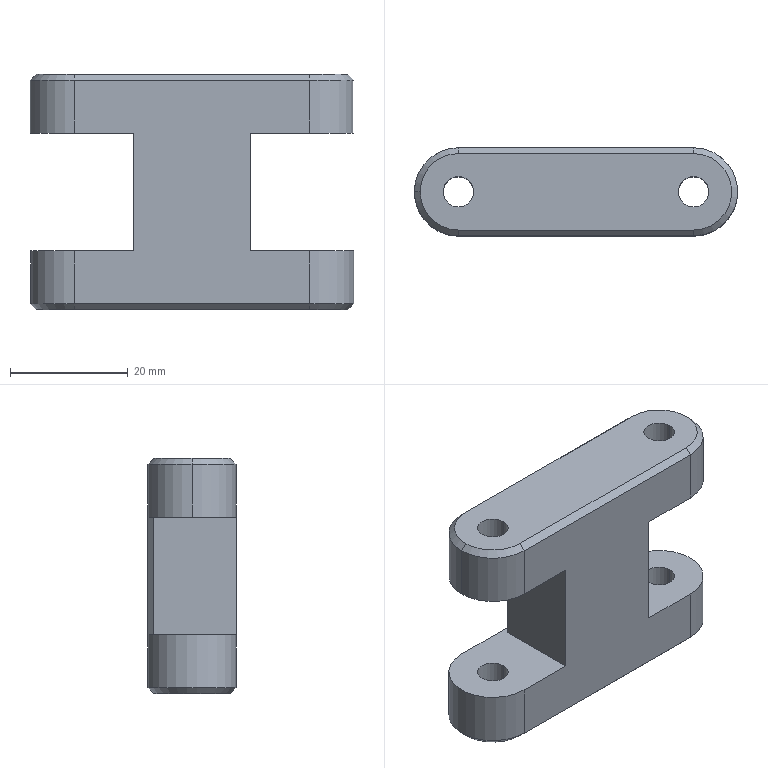Part | SolidWorks | features ICE 2, Chamfer 1, Extrusion 1 | 1 solid | 36 faces | box 55 x 15 x 40 mm | volume 20540 mm3 | plane 16 | cylinder 14 | cone 6 | commonest cylinder face diameters 5.2 x8 15 x6
STEP:
#1=CARTESIAN_POINT('',(-46.5,0.,5.));
#2=VERTEX_POINT('',#1);
#3=CARTESIAN_POINT('',(-40.,-6.5,5.));
#4=VERTEX_POINT('',#3);
#5=CARTESIAN_POINT('',(-40.,0.,5.));
#6=DIRECTION('',(0.,0.,1.));
#7=DIRECTION('',(1.,0.,0.));
#8=AXIS2_PLACEMENT_3D('',#5,#6,#7);
#9=CIRCLE('',#8,6.5);
#10=EDGE_CURVE('',#2,#4,#9,.T.);
#11=ORIENTED_EDGE('',*,*,#10,.F.);
#12=CARTESIAN_POINT('',(-47.5,0.,4.));
#13=VERTEX_POINT('',#12);
#14=CARTESIAN_POINT('',(-46.5,0.,5.));
#15=DIRECTION('',(-0.7071,0.,-0.7071));
#16=VECTOR('',#15,1000.);
#17=LINE('',#14,#16);
#18=EDGE_CURVE('',#2,#13,#17,.T.);
#19=ORIENTED_EDGE('',*,*,#18,.T.);
#20=CARTESIAN_POINT('',(-40.,-7.5,4.));
#21=VERTEX_POINT('',#20);
#22=CARTESIAN_POINT('',(-40.,0.,4.));
#23=DIRECTION('',(0.,0.,-1.));
#24=DIRECTION('',(1.,0.,0.));
#25=AXIS2_PLACEMENT_3D('',#22,#23,#24);
#26=CIRCLE('',#25,7.5);
#27=EDGE_CURVE('',#21,#13,#26,.T.);
#28=ORIENTED_EDGE('',*,*,#27,.F.);
#29=CARTESIAN_POINT('',(-40.,-7.5,4.));
#30=DIRECTION('',(0.,0.7071,0.7071));
#31=VECTOR('',#30,1000.);
#32=LINE('',#29,#31);
#33=EDGE_CURVE('',#21,#4,#32,.T.);
#34=ORIENTED_EDGE('',*,*,#33,.T.);
#35=EDGE_LOOP('',(#11,#19,#28,#34));
#36=FACE_OUTER_BOUND('',#35,.T.);
#37=CARTESIAN_POINT('',(-40.,0.,5.));
#38=DIRECTION('',(0.,0.,-1.));
#39=DIRECTION('',(-1.,0.,0.));
#40=AXIS2_PLACEMENT_3D('',#37,#38,#39);
#41=CONICAL_SURFACE('',#40,6.5,0.7854);
#42=ADVANCED_FACE('',(#36),#41,.T.);
#43=CARTESIAN_POINT('',(6.5,0.,-35.));
#44=VERTEX_POINT('',#43);
#45=CARTESIAN_POINT('',(0.,-6.5,-35.));
#46=VERTEX_POINT('',#45);
#47=CARTESIAN_POINT('',(0.,0.,-35.));
#48=DIRECTION('',(0.,0.,-1.));
#49=DIRECTION('',(-1.,0.,0.));
#50=AXIS2_PLACEMENT_3D('',#47,#48,#49);
#51=CIRCLE('',#50,6.5);
#52=EDGE_CURVE('',#44,#46,#51,.T.);
#53=ORIENTED_EDGE('',*,*,#52,.F.);
#54=CARTESIAN_POINT('',(7.5,0.,-34.));
#55=VERTEX_POINT('',#54);
#56=CARTESIAN_POINT('',(6.5,0.,-35.));
#57=DIRECTION('',(0.7071,0.,0.7071));
#58=VECTOR('',#57,1000.);
#59=LINE('',#56,#58);
#60=EDGE_CURVE('',#44,#55,#59,.T.);
#61=ORIENTED_EDGE('',*,*,#60,.T.);
#62=CARTESIAN_POINT('',(0.,-7.5,-34.));
#63=VERTEX_POINT('',#62);
#64=CARTESIAN_POINT('',(0.,0.,-34.));
#65=DIRECTION('',(0.,0.,1.));
#66=DIRECTION('',(-1.,0.,0.));
#67=AXIS2_PLACEMENT_3D('',#64,#65,#66);
#68=CIRCLE('',#67,7.5);
#69=EDGE_CURVE('',#63,#55,#68,.T.);
#70=ORIENTED_EDGE('',*,*,#69,.F.);
#71=CARTESIAN_POINT('',(0.,-6.5,-35.));
#72=DIRECTION('',(0.,-0.7071,0.7071));
#73=VECTOR('',#72,1000.);
#74=LINE('',#71,#73);
#75=EDGE_CURVE('',#46,#63,#74,.T.);
#76=ORIENTED_EDGE('',*,*,#75,.F.);
#77=EDGE_LOOP('',(#53,#61,#70,#76));
#78=FACE_OUTER_BOUND('',#77,.T.);
#79=CARTESIAN_POINT('',(0.,0.,-35.));
#80=DIRECTION('',(0.,0.,1.));
#81=DIRECTION('',(1.,0.,0.));
#82=AXIS2_PLACEMENT_3D('',#79,#80,#81);
#83=CONICAL_SURFACE('',#82,6.5,0.7854);
#84=ADVANCED_FACE('',(#78),#83,.T.);
#85=CARTESIAN_POINT('',(-37.4,0.,-35.));
#86=VERTEX_POINT('',#85);
#87=CARTESIAN_POINT('',(-42.6,0.,-35.));
#88=VERTEX_POINT('',#87);
#89=CARTESIAN_POINT('',(-40.,0.,-35.));
#90=DIRECTION('',(0.,0.,-1.));
#91=DIRECTION('',(-1.,0.,0.));
#92=AXIS2_PLACEMENT_3D('',#89,#90,#91);
#93=CIRCLE('',#92,2.6);
#94=EDGE_CURVE('',#86,#88,#93,.T.);
#95=ORIENTED_EDGE('',*,*,#94,.T.);
#96=CARTESIAN_POINT('',(-42.6,0.,-25.));
#97=VERTEX_POINT('',#96);
#98=CARTESIAN_POINT('',(-42.6,0.,-35.));
#99=DIRECTION('',(0.,0.,1.));
#100=VECTOR('',#99,1000.);
#101=LINE('',#98,#100);
#102=EDGE_CURVE('',#88,#97,#101,.T.);
#103=ORIENTED_EDGE('',*,*,#102,.T.);
#104=CARTESIAN_POINT('',(-37.4,0.,-25.));
#105=VERTEX_POINT('',#104);
#106=CARTESIAN_POINT('',(-40.,0.,-25.));
#107=DIRECTION('',(0.,0.,-1.));
#108=DIRECTION('',(-1.,0.,0.));
#109=AXIS2_PLACEMENT_3D('',#106,#107,#108);
#110=CIRCLE('',#109,2.6);
#111=EDGE_CURVE('',#105,#97,#110,.T.);
#112=ORIENTED_EDGE('',*,*,#111,.F.);
#113=CARTESIAN_POINT('',(-37.4,0.,-35.));
#114=DIRECTION('',(0.,0.,1.));
#115=VECTOR('',#114,1000.);
#116=LINE('',#113,#115);
#117=EDGE_CURVE('',#86,#105,#116,.T.);
#118=ORIENTED_EDGE('',*,*,#117,.F.);
#119=EDGE_LOOP('',(#95,#103,#112,#118));
#120=FACE_OUTER_BOUND('',#119,.T.);
#121=CARTESIAN_POINT('',(-40.,0.,-35.));
#122=DIRECTION('',(0.,0.,1.));
#123=DIRECTION('',(1.,0.,0.));
#124=AXIS2_PLACEMENT_3D('',#121,#122,#123);
#125=CYLINDRICAL_SURFACE('',#124,2.6);
#126=ADVANCED_FACE('',(#120),#125,.F.);
#127=CARTESIAN_POINT('',(2.6,0.,-35.));
#128=VERTEX_POINT('',#127);
#129=CARTESIAN_POINT('',(-2.6,0.,-35.));
#130=VERTEX_POINT('',#129);
#131=CARTESIAN_POINT('',(0.,0.,-35.));
#132=DIRECTION('',(0.,0.,-1.));
#133=DIRECTION('',(-1.,0.,0.));
#134=AXIS2_PLACEMENT_3D('',#131,#132,#133);
#135=CIRCLE('',#134,2.6);
#136=EDGE_CURVE('',#128,#130,#135,.T.);
#137=ORIENTED_EDGE('',*,*,#136,.T.);
#138=CARTESIAN_POINT('',(-2.6,0.,-25.));
#139=VERTEX_POINT('',#138);
#140=CARTESIAN_POINT('',(-2.6,0.,-35.));
#141=DIRECTION('',(0.,0.,1.));
#142=VECTOR('',#141,1000.);
#143=LINE('',#140,#142);
#144=EDGE_CURVE('',#130,#139,#143,.T.);
#145=ORIENTED_EDGE('',*,*,#144,.T.);
#146=CARTESIAN_POINT('',(2.6,0.,-25.));
#147=VERTEX_POINT('',#146);
#148=CARTESIAN_POINT('',(0.,0.,-25.));
#149=DIRECTION('',(0.,0.,-1.));
#150=DIRECTION('',(-1.,0.,0.));
#151=AXIS2_PLACEMENT_3D('',#148,#149,#150);
#152=CIRCLE('',#151,2.6);
#153=EDGE_CURVE('',#147,#139,#152,.T.);
#154=ORIENTED_EDGE('',*,*,#153,.F.);
#155=CARTESIAN_POINT('',(2.6,0.,-35.));
#156=DIRECTION('',(0.,0.,1.));
#157=VECTOR('',#156,1000.);
#158=LINE('',#155,#157);
#159=EDGE_CURVE('',#128,#147,#158,.T.);
#160=ORIENTED_EDGE('',*,*,#159,.F.);
#161=EDGE_LOOP('',(#137,#145,#154,#160));
#162=FACE_OUTER_BOUND('',#161,.T.);
#163=CARTESIAN_POINT('',(0.,0.,-35.));
#164=DIRECTION('',(0.,0.,1.));
#165=DIRECTION('',(1.,0.,0.));
#166=AXIS2_PLACEMENT_3D('',#163,#164,#165);
#167=CYLINDRICAL_SURFACE('',#166,2.6);
#168=ADVANCED_FACE('',(#162),#167,.F.);
#169=ORIENTED_EDGE('',*,*,#69,.T.);
#170=CARTESIAN_POINT('',(7.5,0.,-25.));
#171=VERTEX_POINT('',#170);
#172=CARTESIAN_POINT('',(7.5,0.,-35.));
#173=DIRECTION('',(0.,0.,1.));
#174=VECTOR('',#173,1000.);
#175=LINE('',#172,#174);
#176=EDGE_CURVE('',#55,#171,#175,.T.);
#177=ORIENTED_EDGE('',*,*,#176,.T.);
#178=CARTESIAN_POINT('',(0.,-7.5,-25.));
#179=VERTEX_POINT('',#178);
#180=CARTESIAN_POINT('',(0.,0.,-25.));
#181=DIRECTION('',(0.,0.,-1.));
#182=DIRECTION('',(-1.,0.,0.));
#183=AXIS2_PLACEMENT_3D('',#180,#181,#182);
#184=CIRCLE('',#183,7.5);
#185=EDGE_CURVE('',#171,#179,#184,.T.);
#186=ORIENTED_EDGE('',*,*,#185,.T.);
#187=CARTESIAN_POINT('',(0.,-7.5,-35.));
#188=DIRECTION('',(0.,0.,1.));
#189=VECTOR('',#188,1000.);
#190=LINE('',#187,#189);
#191=EDGE_CURVE('',#63,#179,#190,.T.);
#192=ORIENTED_EDGE('',*,*,#191,.F.);
#193=EDGE_LOOP('',(#169,#177,#186,#192));
#194=FACE_OUTER_BOUND('',#193,.T.);
#195=CARTESIAN_POINT('',(0.,0.,-35.));
#196=DIRECTION('',(0.,0.,1.));
#197=DIRECTION('',(1.,0.,0.));
#198=AXIS2_PLACEMENT_3D('',#195,#196,#197);
#199=CYLINDRICAL_SURFACE('',#198,7.5);
#200=ADVANCED_FACE('',(#194),#199,.T.);
#201=CARTESIAN_POINT('',(-42.6,0.,5.));
#202=VERTEX_POINT('',#201);
#203=CARTESIAN_POINT('',(-37.4,0.,5.));
#204=VERTEX_POINT('',#203);
#205=CARTESIAN_POINT('',(-40.,0.,5.));
#206=DIRECTION('',(0.,0.,1.));
#207=DIRECTION('',(1.,0.,0.));
#208=AXIS2_PLACEMENT_3D('',#205,#206,#207);
#209=CIRCLE('',#208,2.6);
#210=EDGE_CURVE('',#202,#204,#209,.T.);
#211=ORIENTED_EDGE('',*,*,#210,.T.);
#212=CARTESIAN_POINT('',(-37.4,0.,-5.));
#213=VERTEX_POINT('',#212);
#214=CARTESIAN_POINT('',(-37.4,0.,5.));
#215=DIRECTION('',(0.,0.,-1.));
#216=VECTOR('',#215,1000.);
#217=LINE('',#214,#216);
#218=EDGE_CURVE('',#204,#213,#217,.T.);
#219=ORIENTED_EDGE('',*,*,#218,.T.);
#220=CARTESIAN_POINT('',(-42.6,0.,-5.));
#221=VERTEX_POINT('',#220);
#222=CARTESIAN_POINT('',(-40.,0.,-5.));
#223=DIRECTION('',(0.,0.,1.));
#224=DIRECTION('',(1.,0.,0.));
#225=AXIS2_PLACEMENT_3D('',#222,#223,#224);
#226=CIRCLE('',#225,2.6);
#227=EDGE_CURVE('',#221,#213,#226,.T.);
#228=ORIENTED_EDGE('',*,*,#227,.F.);
#229=CARTESIAN_POINT('',(-42.6,0.,5.));
#230=DIRECTION('',(0.,0.,-1.));
#231=VECTOR('',#230,1000.);
#232=LINE('',#229,#231);
#233=EDGE_CURVE('',#202,#221,#232,.T.);
#234=ORIENTED_EDGE('',*,*,#233,.F.);
#235=EDGE_LOOP('',(#211,#219,#228,#234));
#236=FACE_OUTER_BOUND('',#235,.T.);
#237=CARTESIAN_POINT('',(-40.,0.,5.));
#238=DIRECTION('',(0.,0.,-1.));
#239=DIRECTION('',(-1.,0.,0.));
#240=AXIS2_PLACEMENT_3D('',#237,#238,#239);
#241=CYLINDRICAL_SURFACE('',#240,2.6);
#242=ADVANCED_FACE('',(#236),#241,.F.);
#243=CARTESIAN_POINT('',(-2.6,0.,5.));
#244=VERTEX_POINT('',#243);
#245=CARTESIAN_POINT('',(2.6,0.,5.));
#246=VERTEX_POINT('',#245);
#247=CARTESIAN_POINT('',(0.,0.,5.));
#248=DIRECTION('',(0.,0.,1.));
#249=DIRECTION('',(1.,0.,0.));
#250=AXIS2_PLACEMENT_3D('',#247,#248,#249);
#251=CIRCLE('',#250,2.6);
#252=EDGE_CURVE('',#244,#246,#251,.T.);
#253=ORIENTED_EDGE('',*,*,#252,.T.);
#254=CARTESIAN_POINT('',(2.6,0.,-5.));
#255=VERTEX_POINT('',#254);
#256=CARTESIAN_POINT('',(2.6,0.,5.));
#257=DIRECTION('',(0.,0.,-1.));
#258=VECTOR('',#257,1000.);
#259=LINE('',#256,#258);
#260=EDGE_CURVE('',#246,#255,#259,.T.);
#261=ORIENTED_EDGE('',*,*,#260,.T.);
#262=CARTESIAN_POINT('',(-2.6,0.,-5.));
#263=VERTEX_POINT('',#262);
#264=CARTESIAN_POINT('',(0.,0.,-5.));
#265=DIRECTION('',(0.,0.,1.));
#266=DIRECTION('',(1.,0.,0.));
#267=AXIS2_PLACEMENT_3D('',#264,#265,#266);
#268=CIRCLE('',#267,2.6);
#269=EDGE_CURVE('',#263,#255,#268,.T.);
#270=ORIENTED_EDGE('',*,*,#269,.F.);
#271=CARTESIAN_POINT('',(-2.6,0.,5.));
#272=DIRECTION('',(0.,0.,-1.));
#273=VECTOR('',#272,1000.);
#274=LINE('',#271,#273);
#275=EDGE_CURVE('',#244,#263,#274,.T.);
#276=ORIENTED_EDGE('',*,*,#275,.F.);
#277=EDGE_LOOP('',(#253,#261,#270,#276));
#278=FACE_OUTER_BOUND('',#277,.T.);
#279=CARTESIAN_POINT('',(0.,0.,5.));
#280=DIRECTION('',(0.,0.,-1.));
#281=DIRECTION('',(-1.,0.,0.));
#282=AXIS2_PLACEMENT_3D('',#279,#280,#281);
#283=CYLINDRICAL_SURFACE('',#282,2.6);
#284=ADVANCED_FACE('',(#278),#283,.F.);
#285=ORIENTED_EDGE('',*,*,#27,.T.);
#286=CARTESIAN_POINT('',(-47.5,0.,-5.));
#287=VERTEX_POINT('',#286);
#288=CARTESIAN_POINT('',(-47.5,0.,5.));
#289=DIRECTION('',(0.,0.,-1.));
#290=VECTOR('',#289,1000.);
#291=LINE('',#288,#290);
#292=EDGE_CURVE('',#13,#287,#291,.T.);
#293=ORIENTED_EDGE('',*,*,#292,.T.);
#294=CARTESIAN_POINT('',(-40.,-7.5,-5.));
#295=VERTEX_POINT('',#294);
#296=CARTESIAN_POINT('',(-40.,0.,-5.));
#297=DIRECTION('',(0.,0.,1.));
#298=DIRECTION('',(1.,0.,0.));
#299=AXIS2_PLACEMENT_3D('',#296,#297,#298);
#300=CIRCLE('',#299,7.5);
#301=EDGE_CURVE('',#287,#295,#300,.T.);
#302=ORIENTED_EDGE('',*,*,#301,.T.);
#303=CARTESIAN_POINT('',(-40.,-7.5,5.));
#304=DIRECTION('',(0.,0.,-1.));
#305=VECTOR('',#304,1000.);
#306=LINE('',#303,#305);
#307=EDGE_CURVE('',#21,#295,#306,.T.);
#308=ORIENTED_EDGE('',*,*,#307,.F.);
#309=EDGE_LOOP('',(#285,#293,#302,#308));
#310=FACE_OUTER_BOUND('',#309,.T.);
#311=CARTESIAN_POINT('',(-40.,0.,5.));
#312=DIRECTION('',(0.,0.,-1.));
#313=DIRECTION('',(-1.,0.,0.));
#314=AXIS2_PLACEMENT_3D('',#311,#312,#313);
#315=CYLINDRICAL_SURFACE('',#314,7.5);
#316=ADVANCED_FACE('',(#310),#315,.T.);
#317=ORIENTED_EDGE('',*,*,#227,.T.);
#318=CARTESIAN_POINT('',(-40.,0.,-5.));
#319=DIRECTION('',(0.,0.,1.));
#320=DIRECTION('',(1.,0.,0.));
#321=AXIS2_PLACEMENT_3D('',#318,#319,#320);
#322=CIRCLE('',#321,2.6);
#323=EDGE_CURVE('',#213,#221,#322,.T.);
#324=ORIENTED_EDGE('',*,*,#323,.T.);
#325=EDGE_LOOP('',(#317,#324));
#326=FACE_BOUND('',#325,.T.);
#327=CARTESIAN_POINT('',(-30.,-7.5,-5.));
#328=VERTEX_POINT('',#327);
#329=CARTESIAN_POINT('',(-30.,6.5,-5.));
#330=VERTEX_POINT('',#329);
#331=CARTESIAN_POINT('',(-30.,7.5,-5.));
#332=DIRECTION('',(0.,1.,0.));
#333=VECTOR('',#332,1000.);
#334=LINE('',#331,#333);
#335=EDGE_CURVE('',#328,#330,#334,.T.);
#336=ORIENTED_EDGE('',*,*,#335,.F.);
#337=CARTESIAN_POINT('',(0.,-7.5,-5.));
#338=DIRECTION('',(1.,0.,0.));
#339=VECTOR('',#338,1000.);
#340=LINE('',#337,#339);
#341=EDGE_CURVE('',#295,#328,#340,.T.);
#342=ORIENTED_EDGE('',*,*,#341,.F.);
#343=ORIENTED_EDGE('',*,*,#301,.F.);
#344=CARTESIAN_POINT('',(-40.,7.5,-5.));
#345=VERTEX_POINT('',#344);
#346=CARTESIAN_POINT('',(-40.,0.,-5.));
#347=DIRECTION('',(0.,0.,1.));
#348=DIRECTION('',(1.,0.,0.));
#349=AXIS2_PLACEMENT_3D('',#346,#347,#348);
#350=CIRCLE('',#349,7.5);
#351=EDGE_CURVE('',#345,#287,#350,.T.);
#352=ORIENTED_EDGE('',*,*,#351,.F.);
#353=CARTESIAN_POINT('',(-29.,7.5,-5.));
#354=VERTEX_POINT('',#353);
#355=CARTESIAN_POINT('',(0.,7.5,-5.));
#356=DIRECTION('',(-1.,0.,0.));
#357=VECTOR('',#356,1000.);
#358=LINE('',#355,#357);
#359=EDGE_CURVE('',#354,#345,#358,.T.);
#360=ORIENTED_EDGE('',*,*,#359,.F.);
#361=CARTESIAN_POINT('',(-18.25,18.25,-5.));
#362=DIRECTION('',(-0.7071,-0.7071,0.));
#363=VECTOR('',#362,1000.);
#364=LINE('',#361,#363);
#365=EDGE_CURVE('',#354,#330,#364,.T.);
#366=ORIENTED_EDGE('',*,*,#365,.T.);
#367=EDGE_LOOP('',(#336,#342,#343,#352,#360,#366));
#368=FACE_OUTER_BOUND('',#367,.T.);
#369=CARTESIAN_POINT('',(0.,0.,-5.));
#370=DIRECTION('',(0.,0.,1.));
#371=DIRECTION('',(1.,0.,0.));
#372=AXIS2_PLACEMENT_3D('',#369,#370,#371);
#373=PLANE('',#372);
#374=ADVANCED_FACE('',(#326,#368),#373,.F.);
#375=ORIENTED_EDGE('',*,*,#269,.T.);
#376=CARTESIAN_POINT('',(0.,0.,-5.));
#377=DIRECTION('',(0.,0.,1.));
#378=DIRECTION('',(1.,0.,0.));
#379=AXIS2_PLACEMENT_3D('',#376,#377,#378);
#380=CIRCLE('',#379,2.6);
#381=EDGE_CURVE('',#255,#263,#380,.T.);
#382=ORIENTED_EDGE('',*,*,#381,.T.);
#383=EDGE_LOOP('',(#375,#382));
#384=FACE_BOUND('',#383,.T.);
#385=CARTESIAN_POINT('',(-10.,6.5,-5.));
#386=VERTEX_POINT('',#385);
#387=CARTESIAN_POINT('',(-10.,-7.5,-5.));
#388=VERTEX_POINT('',#387);
#389=CARTESIAN_POINT('',(-10.,7.5,-5.));
#390=DIRECTION('',(0.,-1.,0.));
#391=VECTOR('',#390,1000.);
#392=LINE('',#389,#391);
#393=EDGE_CURVE('',#386,#388,#392,.T.);
#394=ORIENTED_EDGE('',*,*,#393,.F.);
#395=CARTESIAN_POINT('',(-11.,7.5,-5.));
#396=VERTEX_POINT('',#395);
#397=CARTESIAN_POINT('',(-1.75,-1.75,-5.));
#398=DIRECTION('',(-0.7071,0.7071,0.));
#399=VECTOR('',#398,1000.);
#400=LINE('',#397,#399);
#401=EDGE_CURVE('',#386,#396,#400,.T.);
#402=ORIENTED_EDGE('',*,*,#401,.T.);
#403=CARTESIAN_POINT('',(0.,7.5,-5.));
#404=VERTEX_POINT('',#403);
#405=CARTESIAN_POINT('',(0.,7.5,-5.));
#406=DIRECTION('',(-1.,0.,0.));
#407=VECTOR('',#406,1000.);
#408=LINE('',#405,#407);
#409=EDGE_CURVE('',#404,#396,#408,.T.);
#410=ORIENTED_EDGE('',*,*,#409,.F.);
#411=CARTESIAN_POINT('',(0.,-7.5,-5.));
#412=VERTEX_POINT('',#411);
#413=CARTESIAN_POINT('',(0.,0.,-5.));
#414=DIRECTION('',(0.,0.,1.));
#415=DIRECTION('',(1.,0.,0.));
#416=AXIS2_PLACEMENT_3D('',#413,#414,#415);
#417=CIRCLE('',#416,7.5);
#418=EDGE_CURVE('',#412,#404,#417,.T.);
#419=ORIENTED_EDGE('',*,*,#418,.F.);
#420=CARTESIAN_POINT('',(0.,-7.5,-5.));
#421=DIRECTION('',(1.,0.,0.));
#422=VECTOR('',#421,1000.);
#423=LINE('',#420,#422);
#424=EDGE_CURVE('',#388,#412,#423,.T.);
#425=ORIENTED_EDGE('',*,*,#424,.F.);
#426=EDGE_LOOP('',(#394,#402,#410,#419,#425));
#427=FACE_OUTER_BOUND('',#426,.T.);
#428=CARTESIAN_POINT('',(0.,0.,-5.));
#429=DIRECTION('',(0.,0.,1.));
#430=DIRECTION('',(1.,0.,0.));
#431=AXIS2_PLACEMENT_3D('',#428,#429,#430);
#432=PLANE('',#431);
#433=ADVANCED_FACE('',(#384,#427),#432,.F.);
#434=CARTESIAN_POINT('',(0.,6.5,5.));
#435=VERTEX_POINT('',#434);
#436=CARTESIAN_POINT('',(-40.,6.5,5.));
#437=VERTEX_POINT('',#436);
#438=CARTESIAN_POINT('',(-40.,6.5,5.));
#439=DIRECTION('',(-1.,0.,0.));
#440=VECTOR('',#439,1000.);
#441=LINE('',#438,#440);
#442=EDGE_CURVE('',#435,#437,#441,.T.);
#443=ORIENTED_EDGE('',*,*,#442,.T.);
#444=CARTESIAN_POINT('',(-40.,0.,5.));
#445=DIRECTION('',(0.,0.,1.));
#446=DIRECTION('',(1.,0.,0.));
#447=AXIS2_PLACEMENT_3D('',#444,#445,#446);
#448=CIRCLE('',#447,6.5);
#449=EDGE_CURVE('',#437,#2,#448,.T.);
#450=ORIENTED_EDGE('',*,*,#449,.T.);
#451=ORIENTED_EDGE('',*,*,#10,.T.);
#452=CARTESIAN_POINT('',(0.,-6.5,5.));
#453=VERTEX_POINT('',#452);
#454=CARTESIAN_POINT('',(0.,-6.5,5.));
#455=DIRECTION('',(1.,0.,0.));
#456=VECTOR('',#455,1000.);
#457=LINE('',#454,#456);
#458=EDGE_CURVE('',#4,#453,#457,.T.);
#459=ORIENTED_EDGE('',*,*,#458,.T.);
#460=CARTESIAN_POINT('',(0.,0.,5.));
#461=DIRECTION('',(0.,0.,1.));
#462=DIRECTION('',(1.,0.,0.));
#463=AXIS2_PLACEMENT_3D('',#460,#461,#462);
#464=CIRCLE('',#463,6.5);
#465=EDGE_CURVE('',#453,#435,#464,.T.);
#466=ORIENTED_EDGE('',*,*,#465,.T.);
#467=EDGE_LOOP('',(#443,#450,#451,#459,#466));
#468=FACE_OUTER_BOUND('',#467,.T.);
#469=ORIENTED_EDGE('',*,*,#252,.F.);
#470=CARTESIAN_POINT('',(0.,0.,5.));
#471=DIRECTION('',(0.,0.,1.));
#472=DIRECTION('',(1.,0.,0.));
#473=AXIS2_PLACEMENT_3D('',#470,#471,#472);
#474=CIRCLE('',#473,2.6);
#475=EDGE_CURVE('',#246,#244,#474,.T.);
#476=ORIENTED_EDGE('',*,*,#475,.F.);
#477=EDGE_LOOP('',(#469,#476));
#478=FACE_BOUND('',#477,.T.);
#479=ORIENTED_EDGE('',*,*,#210,.F.);
#480=CARTESIAN_POINT('',(-40.,0.,5.));
#481=DIRECTION('',(0.,0.,1.));
#482=DIRECTION('',(1.,0.,0.));
#483=AXIS2_PLACEMENT_3D('',#480,#481,#482);
#484=CIRCLE('',#483,2.6);
#485=EDGE_CURVE('',#204,#202,#484,.T.);
#486=ORIENTED_EDGE('',*,*,#485,.F.);
#487=EDGE_LOOP('',(#479,#486));
#488=FACE_BOUND('',#487,.T.);
#489=CARTESIAN_POINT('',(0.,0.,5.));
#490=DIRECTION('',(0.,0.,1.));
#491=DIRECTION('',(1.,0.,0.));
#492=AXIS2_PLACEMENT_3D('',#489,#490,#491);
#493=PLANE('',#492);
#494=ADVANCED_FACE('',(#468,#478,#488),#493,.T.);
#495=CARTESIAN_POINT('',(0.,7.5,4.));
#496=VERTEX_POINT('',#495);
#497=CARTESIAN_POINT('',(0.,7.5,5.));
#498=DIRECTION('',(0.,0.,-1.));
#499=VECTOR('',#498,1000.);
#500=LINE('',#497,#499);
#501=EDGE_CURVE('',#496,#404,#500,.T.);
#502=ORIENTED_EDGE('',*,*,#501,.F.);
#503=CARTESIAN_POINT('',(0.,-7.5,4.));
#504=VERTEX_POINT('',#503);
#505=CARTESIAN_POINT('',(0.,0.,4.));
#506=DIRECTION('',(0.,0.,-1.));
#507=DIRECTION('',(1.,0.,0.));
#508=AXIS2_PLACEMENT_3D('',#505,#506,#507);
#509=CIRCLE('',#508,7.5);
#510=EDGE_CURVE('',#496,#504,#509,.T.);
#511=ORIENTED_EDGE('',*,*,#510,.T.);
#512=CARTESIAN_POINT('',(0.,-7.5,5.));
#513=DIRECTION('',(0.,0.,-1.));
#514=VECTOR('',#513,1000.);
#515=LINE('',#512,#514);
#516=EDGE_CURVE('',#504,#412,#515,.T.);
#517=ORIENTED_EDGE('',*,*,#516,.T.);
#518=ORIENTED_EDGE('',*,*,#418,.T.);
#519=EDGE_LOOP('',(#502,#511,#517,#518));
#520=FACE_OUTER_BOUND('',#519,.T.);
#521=CARTESIAN_POINT('',(0.,0.,5.));
#522=DIRECTION('',(0.,0.,-1.));
#523=DIRECTION('',(-1.,0.,0.));
#524=AXIS2_PLACEMENT_3D('',#521,#522,#523);
#525=CYLINDRICAL_SURFACE('',#524,7.5);
#526=ADVANCED_FACE('',(#520),#525,.T.);
#527=ORIENTED_EDGE('',*,*,#409,.T.);
#528=CARTESIAN_POINT('',(-11.,7.5,-25.));
#529=VERTEX_POINT('',#528);
#530=CARTESIAN_POINT('',(-11.,7.5,5.));
#531=DIRECTION('',(0.,0.,-1.));
#532=VECTOR('',#531,1000.);
#533=LINE('',#530,#532);
#534=EDGE_CURVE('',#396,#529,#533,.T.);
#535=ORIENTED_EDGE('',*,*,#534,.T.);
#536=CARTESIAN_POINT('',(0.,7.5,-25.));
#537=VERTEX_POINT('',#536);
#538=CARTESIAN_POINT('',(0.,7.5,-25.));
#539=DIRECTION('',(1.,0.,0.));
#540=VECTOR('',#539,1000.);
#541=LINE('',#538,#540);
#542=EDGE_CURVE('',#529,#537,#541,.T.);
#543=ORIENTED_EDGE('',*,*,#542,.T.);
#544=CARTESIAN_POINT('',(0.,7.5,-34.));
#545=VERTEX_POINT('',#544);
#546=CARTESIAN_POINT('',(0.,7.5,-35.));
#547=DIRECTION('',(0.,0.,1.));
#548=VECTOR('',#547,1000.);
#549=LINE('',#546,#548);
#550=EDGE_CURVE('',#545,#537,#549,.T.);
#551=ORIENTED_EDGE('',*,*,#550,.F.);
#552=CARTESIAN_POINT('',(-40.,7.5,-34.));
#553=VERTEX_POINT('',#552);
#554=CARTESIAN_POINT('',(-40.,7.5,-34.));
#555=DIRECTION('',(-1.,0.,0.));
#556=VECTOR('',#555,1000.);
#557=LINE('',#554,#556);
#558=EDGE_CURVE('',#545,#553,#557,.T.);
#559=ORIENTED_EDGE('',*,*,#558,.T.);
#560=CARTESIAN_POINT('',(-40.,7.5,-25.));
#561=VERTEX_POINT('',#560);
#562=CARTESIAN_POINT('',(-40.,7.5,-35.));
#563=DIRECTION('',(0.,0.,1.));
#564=VECTOR('',#563,1000.);
#565=LINE('',#562,#564);
#566=EDGE_CURVE('',#553,#561,#565,.T.);
#567=ORIENTED_EDGE('',*,*,#566,.T.);
#568=CARTESIAN_POINT('',(-29.,7.5,-25.));
#569=VERTEX_POINT('',#568);
#570=CARTESIAN_POINT('',(0.,7.5,-25.));
#571=DIRECTION('',(1.,0.,0.));
#572=VECTOR('',#571,1000.);
#573=LINE('',#570,#572);
#574=EDGE_CURVE('',#561,#569,#573,.T.);
#575=ORIENTED_EDGE('',*,*,#574,.T.);
#576=CARTESIAN_POINT('',(-29.,7.5,5.));
#577=DIRECTION('',(0.,0.,1.));
#578=VECTOR('',#577,1000.);
#579=LINE('',#576,#578);
#580=EDGE_CURVE('',#569,#354,#579,.T.);
#581=ORIENTED_EDGE('',*,*,#580,.T.);
#582=ORIENTED_EDGE('',*,*,#359,.T.);
#583=CARTESIAN_POINT('',(-40.,7.5,4.));
#584=VERTEX_POINT('',#583);
#585=CARTESIAN_POINT('',(-40.,7.5,5.));
#586=DIRECTION('',(0.,0.,-1.));
#587=VECTOR('',#586,1000.);
#588=LINE('',#585,#587);
#589=EDGE_CURVE('',#584,#345,#588,.T.);
#590=ORIENTED_EDGE('',*,*,#589,.F.);
#591=CARTESIAN_POINT('',(0.,7.5,4.));
#592=DIRECTION('',(1.,0.,0.));
#593=VECTOR('',#592,1000.);
#594=LINE('',#591,#593);
#595=EDGE_CURVE('',#584,#496,#594,.T.);
#596=ORIENTED_EDGE('',*,*,#595,.T.);
#597=ORIENTED_EDGE('',*,*,#501,.T.);
#598=EDGE_LOOP('',(#527,#535,#543,#551,#559,#567,#575,#581,#582,#590,#596,#597));
#599=FACE_OUTER_BOUND('',#598,.T.);
#600=CARTESIAN_POINT('',(0.,7.5,5.));
#601=DIRECTION('',(0.,-1.,0.));
#602=DIRECTION('',(1.,0.,0.));
#603=AXIS2_PLACEMENT_3D('',#600,#601,#602);
#604=PLANE('',#603);
#605=ADVANCED_FACE('',(#599),#604,.F.);
#606=ORIENTED_EDGE('',*,*,#292,.F.);
#607=CARTESIAN_POINT('',(-40.,0.,4.));
#608=DIRECTION('',(0.,0.,-1.));
#609=DIRECTION('',(1.,0.,0.));
#610=AXIS2_PLACEMENT_3D('',#607,#608,#609);
#611=CIRCLE('',#610,7.5);
#612=EDGE_CURVE('',#13,#584,#611,.T.);
#613=ORIENTED_EDGE('',*,*,#612,.T.);
#614=ORIENTED_EDGE('',*,*,#589,.T.);
#615=ORIENTED_EDGE('',*,*,#351,.T.);
#616=EDGE_LOOP('',(#606,#613,#614,#615));
#617=FACE_OUTER_BOUND('',#616,.T.);
#618=CARTESIAN_POINT('',(-40.,0.,5.));
#619=DIRECTION('',(0.,0.,-1.));
#620=DIRECTION('',(-1.,0.,0.));
#621=AXIS2_PLACEMENT_3D('',#618,#619,#620);
#622=CYLINDRICAL_SURFACE('',#621,7.5);
#623=ADVANCED_FACE('',(#617),#622,.T.);
#624=CARTESIAN_POINT('',(-40.,-7.5,-34.));
#625=VERTEX_POINT('',#624);
#626=CARTESIAN_POINT('',(-40.,-7.5,-25.));
#627=VERTEX_POINT('',#626);
#628=CARTESIAN_POINT('',(-40.,-7.5,-35.));
#629=DIRECTION('',(0.,0.,1.));
#630=VECTOR('',#629,1000.);
#631=LINE('',#628,#630);
#632=EDGE_CURVE('',#625,#627,#631,.T.);
#633=ORIENTED_EDGE('',*,*,#632,.F.);
#634=CARTESIAN_POINT('',(0.,-7.5,-34.));
#635=DIRECTION('',(1.,0.,0.));
#636=VECTOR('',#635,1000.);
#637=LINE('',#634,#636);
#638=EDGE_CURVE('',#625,#63,#637,.T.);
#639=ORIENTED_EDGE('',*,*,#638,.T.);
#640=ORIENTED_EDGE('',*,*,#191,.T.);
#641=CARTESIAN_POINT('',(-10.,-7.5,-25.));
#642=VERTEX_POINT('',#641);
#643=CARTESIAN_POINT('',(0.,-7.5,-25.));
#644=DIRECTION('',(-1.,0.,0.));
#645=VECTOR('',#644,1000.);
#646=LINE('',#643,#645);
#647=EDGE_CURVE('',#179,#642,#646,.T.);
#648=ORIENTED_EDGE('',*,*,#647,.T.);
#649=CARTESIAN_POINT('',(-10.,-7.5,-25.));
#650=DIRECTION('',(0.,0.,1.));
#651=VECTOR('',#650,1000.);
#652=LINE('',#649,#651);
#653=EDGE_CURVE('',#642,#388,#652,.T.);
#654=ORIENTED_EDGE('',*,*,#653,.T.);
#655=ORIENTED_EDGE('',*,*,#424,.T.);
#656=ORIENTED_EDGE('',*,*,#516,.F.);
#657=CARTESIAN_POINT('',(-40.,-7.5,4.));
#658=DIRECTION('',(-1.,0.,0.));
#659=VECTOR('',#658,1000.);
#660=LINE('',#657,#659);
#661=EDGE_CURVE('',#504,#21,#660,.T.);
#662=ORIENTED_EDGE('',*,*,#661,.T.);
#663=ORIENTED_EDGE('',*,*,#307,.T.);
#664=ORIENTED_EDGE('',*,*,#341,.T.);
#665=CARTESIAN_POINT('',(-30.,-7.5,-25.));
#666=VERTEX_POINT('',#665);
#667=CARTESIAN_POINT('',(-30.,-7.5,-25.));
#668=DIRECTION('',(0.,0.,1.));
#669=VECTOR('',#668,1000.);
#670=LINE('',#667,#669);
#671=EDGE_CURVE('',#666,#328,#670,.T.);
#672=ORIENTED_EDGE('',*,*,#671,.F.);
#673=CARTESIAN_POINT('',(0.,-7.5,-25.));
#674=DIRECTION('',(-1.,0.,0.));
#675=VECTOR('',#674,1000.);
#676=LINE('',#673,#675);
#677=EDGE_CURVE('',#666,#627,#676,.T.);
#678=ORIENTED_EDGE('',*,*,#677,.T.);
#679=EDGE_LOOP('',(#633,#639,#640,#648,#654,#655,#656,#662,#663,#664,#672,#678));
#680=FACE_OUTER_BOUND('',#679,.T.);
#681=CARTESIAN_POINT('',(0.,-7.5,5.));
#682=DIRECTION('',(0.,1.,0.));
#683=DIRECTION('',(-1.,0.,0.));
#684=AXIS2_PLACEMENT_3D('',#681,#682,#683);
#685=PLANE('',#684);
#686=ADVANCED_FACE('',(#680),#685,.F.);
#687=ORIENTED_EDGE('',*,*,#260,.F.);
#688=ORIENTED_EDGE('',*,*,#475,.T.);
#689=ORIENTED_EDGE('',*,*,#275,.T.);
#690=ORIENTED_EDGE('',*,*,#381,.F.);
#691=EDGE_LOOP('',(#687,#688,#689,#690));
#692=FACE_OUTER_BOUND('',#691,.T.);
#693=CARTESIAN_POINT('',(0.,0.,5.));
#694=DIRECTION('',(0.,0.,-1.));
#695=DIRECTION('',(-1.,0.,0.));
#696=AXIS2_PLACEMENT_3D('',#693,#694,#695);
#697=CYLINDRICAL_SURFACE('',#696,2.6);
#698=ADVANCED_FACE('',(#692),#697,.F.);
#699=ORIENTED_EDGE('',*,*,#218,.F.);
#700=ORIENTED_EDGE('',*,*,#485,.T.);
#701=ORIENTED_EDGE('',*,*,#233,.T.);
#702=ORIENTED_EDGE('',*,*,#323,.F.);
#703=EDGE_LOOP('',(#699,#700,#701,#702));
#704=FACE_OUTER_BOUND('',#703,.T.);
#705=CARTESIAN_POINT('',(-40.,0.,5.));
#706=DIRECTION('',(0.,0.,-1.));
#707=DIRECTION('',(-1.,0.,0.));
#708=AXIS2_PLACEMENT_3D('',#705,#706,#707);
#709=CYLINDRICAL_SURFACE('',#708,2.6);
#710=ADVANCED_FACE('',(#704),#709,.F.);
#711=ORIENTED_EDGE('',*,*,#335,.T.);
#712=CARTESIAN_POINT('',(-30.,6.5,-25.));
#713=VERTEX_POINT('',#712);
#714=CARTESIAN_POINT('',(-30.,6.5,-25.));
#715=DIRECTION('',(0.,0.,-1.));
#716=VECTOR('',#715,1000.);
#717=LINE('',#714,#716);
#718=EDGE_CURVE('',#330,#713,#717,.T.);
#719=ORIENTED_EDGE('',*,*,#718,.T.);
#720=CARTESIAN_POINT('',(-30.,7.5,-25.));
#721=DIRECTION('',(0.,1.,0.));
#722=VECTOR('',#721,1000.);
#723=LINE('',#720,#722);
#724=EDGE_CURVE('',#666,#713,#723,.T.);
#725=ORIENTED_EDGE('',*,*,#724,.F.);
#726=ORIENTED_EDGE('',*,*,#671,.T.);
#727=EDGE_LOOP('',(#711,#719,#725,#726));
#728=FACE_OUTER_BOUND('',#727,.T.);
#729=CARTESIAN_POINT('',(-30.,7.5,-25.));
#730=DIRECTION('',(1.,0.,0.));
#731=DIRECTION('',(0.,0.,-1.));
#732=AXIS2_PLACEMENT_3D('',#729,#730,#731);
#733=PLANE('',#732);
#734=ADVANCED_FACE('',(#728),#733,.F.);
#735=CARTESIAN_POINT('',(-10.,6.5,-25.));
#736=VERTEX_POINT('',#735);
#737=CARTESIAN_POINT('',(-10.,7.5,-25.));
#738=DIRECTION('',(0.,-1.,0.));
#739=VECTOR('',#738,1000.);
#740=LINE('',#737,#739);
#741=EDGE_CURVE('',#736,#642,#740,.T.);
#742=ORIENTED_EDGE('',*,*,#741,.F.);
#743=CARTESIAN_POINT('',(-10.,6.5,-25.));
#744=DIRECTION('',(0.,0.,1.));
#745=VECTOR('',#744,1000.);
#746=LINE('',#743,#745);
#747=EDGE_CURVE('',#736,#386,#746,.T.);
#748=ORIENTED_EDGE('',*,*,#747,.T.);
#749=ORIENTED_EDGE('',*,*,#393,.T.);
#750=ORIENTED_EDGE('',*,*,#653,.F.);
#751=EDGE_LOOP('',(#742,#748,#749,#750));
#752=FACE_OUTER_BOUND('',#751,.T.);
#753=CARTESIAN_POINT('',(-10.,7.5,-25.));
#754=DIRECTION('',(-1.,0.,0.));
#755=DIRECTION('',(0.,0.,1.));
#756=AXIS2_PLACEMENT_3D('',#753,#754,#755);
#757=PLANE('',#756);
#758=ADVANCED_FACE('',(#752),#757,.F.);
#759=ORIENTED_EDGE('',*,*,#111,.T.);
#760=CARTESIAN_POINT('',(-40.,0.,-25.));
#761=DIRECTION('',(0.,0.,-1.));
#762=DIRECTION('',(-1.,0.,0.));
#763=AXIS2_PLACEMENT_3D('',#760,#761,#762);
#764=CIRCLE('',#763,2.6);
#765=EDGE_CURVE('',#97,#105,#764,.T.);
#766=ORIENTED_EDGE('',*,*,#765,.T.);
#767=EDGE_LOOP('',(#759,#766));
#768=FACE_BOUND('',#767,.T.);
#769=ORIENTED_EDGE('',*,*,#677,.F.);
#770=ORIENTED_EDGE('',*,*,#724,.T.);
#771=CARTESIAN_POINT('',(-18.25,18.25,-25.));
#772=DIRECTION('',(0.7071,0.7071,0.));
#773=VECTOR('',#772,1000.);
#774=LINE('',#771,#773);
#775=EDGE_CURVE('',#713,#569,#774,.T.);
#776=ORIENTED_EDGE('',*,*,#775,.T.);
#777=ORIENTED_EDGE('',*,*,#574,.F.);
#778=CARTESIAN_POINT('',(-40.,0.,-25.));
#779=DIRECTION('',(0.,0.,-1.));
#780=DIRECTION('',(-1.,0.,0.));
#781=AXIS2_PLACEMENT_3D('',#778,#779,#780);
#782=CIRCLE('',#781,7.5);
#783=EDGE_CURVE('',#627,#561,#782,.T.);
#784=ORIENTED_EDGE('',*,*,#783,.F.);
#785=EDGE_LOOP('',(#769,#770,#776,#777,#784));
#786=FACE_OUTER_BOUND('',#785,.T.);
#787=CARTESIAN_POINT('',(0.,0.,-25.));
#788=DIRECTION('',(0.,0.,-1.));
#789=DIRECTION('',(-1.,0.,0.));
#790=AXIS2_PLACEMENT_3D('',#787,#788,#789);
#791=PLANE('',#790);
#792=ADVANCED_FACE('',(#768,#786),#791,.F.);
#793=ORIENTED_EDGE('',*,*,#153,.T.);
#794=CARTESIAN_POINT('',(0.,0.,-25.));
#795=DIRECTION('',(0.,0.,-1.));
#796=DIRECTION('',(-1.,0.,0.));
#797=AXIS2_PLACEMENT_3D('',#794,#795,#796);
#798=CIRCLE('',#797,2.6);
#799=EDGE_CURVE('',#139,#147,#798,.T.);
#800=ORIENTED_EDGE('',*,*,#799,.T.);
#801=EDGE_LOOP('',(#793,#800));
#802=FACE_BOUND('',#801,.T.);
#803=ORIENTED_EDGE('',*,*,#542,.F.);
#804=CARTESIAN_POINT('',(-1.75,-1.75,-25.));
#805=DIRECTION('',(0.7071,-0.7071,0.));
#806=VECTOR('',#805,1000.);
#807=LINE('',#804,#806);
#808=EDGE_CURVE('',#529,#736,#807,.T.);
#809=ORIENTED_EDGE('',*,*,#808,.T.);
#810=ORIENTED_EDGE('',*,*,#741,.T.);
#811=ORIENTED_EDGE('',*,*,#647,.F.);
#812=ORIENTED_EDGE('',*,*,#185,.F.);
#813=CARTESIAN_POINT('',(0.,0.,-25.));
#814=DIRECTION('',(0.,0.,-1.));
#815=DIRECTION('',(-1.,0.,0.));
#816=AXIS2_PLACEMENT_3D('',#813,#814,#815);
#817=CIRCLE('',#816,7.5);
#818=EDGE_CURVE('',#537,#171,#817,.T.);
#819=ORIENTED_EDGE('',*,*,#818,.F.);
#820=EDGE_LOOP('',(#803,#809,#810,#811,#812,#819));
#821=FACE_OUTER_BOUND('',#820,.T.);
#822=CARTESIAN_POINT('',(0.,0.,-25.));
#823=DIRECTION('',(0.,0.,-1.));
#824=DIRECTION('',(-1.,0.,0.));
#825=AXIS2_PLACEMENT_3D('',#822,#823,#824);
#826=PLANE('',#825);
#827=ADVANCED_FACE('',(#802,#821),#826,.F.);
#828=CARTESIAN_POINT('',(-40.,-6.5,-35.));
#829=VERTEX_POINT('',#828);
#830=CARTESIAN_POINT('',(-40.,-6.5,-35.));
#831=DIRECTION('',(-1.,0.,0.));
#832=VECTOR('',#831,1000.);
#833=LINE('',#830,#832);
#834=EDGE_CURVE('',#46,#829,#833,.T.);
#835=ORIENTED_EDGE('',*,*,#834,.T.);
#836=CARTESIAN_POINT('',(-40.,6.5,-35.));
#837=VERTEX_POINT('',#836);
#838=CARTESIAN_POINT('',(-40.,0.,-35.));
#839=DIRECTION('',(0.,0.,-1.));
#840=DIRECTION('',(-1.,0.,0.));
#841=AXIS2_PLACEMENT_3D('',#838,#839,#840);
#842=CIRCLE('',#841,6.5);
#843=EDGE_CURVE('',#829,#837,#842,.T.);
#844=ORIENTED_EDGE('',*,*,#843,.T.);
#845=CARTESIAN_POINT('',(0.,6.5,-35.));
#846=VERTEX_POINT('',#845);
#847=CARTESIAN_POINT('',(0.,6.5,-35.));
#848=DIRECTION('',(1.,0.,0.));
#849=VECTOR('',#848,1000.);
#850=LINE('',#847,#849);
#851=EDGE_CURVE('',#837,#846,#850,.T.);
#852=ORIENTED_EDGE('',*,*,#851,.T.);
#853=CARTESIAN_POINT('',(0.,0.,-35.));
#854=DIRECTION('',(0.,0.,-1.));
#855=DIRECTION('',(-1.,0.,0.));
#856=AXIS2_PLACEMENT_3D('',#853,#854,#855);
#857=CIRCLE('',#856,6.5);
#858=EDGE_CURVE('',#846,#44,#857,.T.);
#859=ORIENTED_EDGE('',*,*,#858,.T.);
#860=ORIENTED_EDGE('',*,*,#52,.T.);
#861=EDGE_LOOP('',(#835,#844,#852,#859,#860));
#862=FACE_OUTER_BOUND('',#861,.T.);
#863=ORIENTED_EDGE('',*,*,#136,.F.);
#864=CARTESIAN_POINT('',(0.,0.,-35.));
#865=DIRECTION('',(0.,0.,-1.));
#866=DIRECTION('',(-1.,0.,0.));
#867=AXIS2_PLACEMENT_3D('',#864,#865,#866);
#868=CIRCLE('',#867,2.6);
#869=EDGE_CURVE('',#130,#128,#868,.T.);
#870=ORIENTED_EDGE('',*,*,#869,.F.);
#871=EDGE_LOOP('',(#863,#870));
#872=FACE_BOUND('',#871,.T.);
#873=ORIENTED_EDGE('',*,*,#94,.F.);
#874=CARTESIAN_POINT('',(-40.,0.,-35.));
#875=DIRECTION('',(0.,0.,-1.));
#876=DIRECTION('',(-1.,0.,0.));
#877=AXIS2_PLACEMENT_3D('',#874,#875,#876);
#878=CIRCLE('',#877,2.6);
#879=EDGE_CURVE('',#88,#86,#878,.T.);
#880=ORIENTED_EDGE('',*,*,#879,.F.);
#881=EDGE_LOOP('',(#873,#880));
#882=FACE_BOUND('',#881,.T.);
#883=CARTESIAN_POINT('',(0.,0.,-35.));
#884=DIRECTION('',(0.,0.,-1.));
#885=DIRECTION('',(-1.,0.,0.));
#886=AXIS2_PLACEMENT_3D('',#883,#884,#885);
#887=PLANE('',#886);
#888=ADVANCED_FACE('',(#862,#872,#882),#887,.T.);
#889=ORIENTED_EDGE('',*,*,#176,.F.);
#890=CARTESIAN_POINT('',(0.,0.,-34.));
#891=DIRECTION('',(0.,0.,1.));
#892=DIRECTION('',(-1.,0.,0.));
#893=AXIS2_PLACEMENT_3D('',#890,#891,#892);
#894=CIRCLE('',#893,7.5);
#895=EDGE_CURVE('',#55,#545,#894,.T.);
#896=ORIENTED_EDGE('',*,*,#895,.T.);
#897=ORIENTED_EDGE('',*,*,#550,.T.);
#898=ORIENTED_EDGE('',*,*,#818,.T.);
#899=EDGE_LOOP('',(#889,#896,#897,#898));
#900=FACE_OUTER_BOUND('',#899,.T.);
#901=CARTESIAN_POINT('',(0.,0.,-35.));
#902=DIRECTION('',(0.,0.,1.));
#903=DIRECTION('',(1.,0.,0.));
#904=AXIS2_PLACEMENT_3D('',#901,#902,#903);
#905=CYLINDRICAL_SURFACE('',#904,7.5);
#906=ADVANCED_FACE('',(#900),#905,.T.);
#907=ORIENTED_EDGE('',*,*,#566,.F.);
#908=CARTESIAN_POINT('',(-40.,0.,-34.));
#909=DIRECTION('',(0.,0.,1.));
#910=DIRECTION('',(-1.,0.,0.));
#911=AXIS2_PLACEMENT_3D('',#908,#909,#910);
#912=CIRCLE('',#911,7.5);
#913=EDGE_CURVE('',#553,#625,#912,.T.);
#914=ORIENTED_EDGE('',*,*,#913,.T.);
#915=ORIENTED_EDGE('',*,*,#632,.T.);
#916=ORIENTED_EDGE('',*,*,#783,.T.);
#917=EDGE_LOOP('',(#907,#914,#915,#916));
#918=FACE_OUTER_BOUND('',#917,.T.);
#919=CARTESIAN_POINT('',(-40.,0.,-35.));
#920=DIRECTION('',(0.,0.,1.));
#921=DIRECTION('',(1.,0.,0.));
#922=AXIS2_PLACEMENT_3D('',#919,#920,#921);
#923=CYLINDRICAL_SURFACE('',#922,7.5);
#924=ADVANCED_FACE('',(#918),#923,.T.);
#925=ORIENTED_EDGE('',*,*,#144,.F.);
#926=ORIENTED_EDGE('',*,*,#869,.T.);
#927=ORIENTED_EDGE('',*,*,#159,.T.);
#928=ORIENTED_EDGE('',*,*,#799,.F.);
#929=EDGE_LOOP('',(#925,#926,#927,#928));
#930=FACE_OUTER_BOUND('',#929,.T.);
#931=CARTESIAN_POINT('',(0.,0.,-35.));
#932=DIRECTION('',(0.,0.,1.));
#933=DIRECTION('',(1.,0.,0.));
#934=AXIS2_PLACEMENT_3D('',#931,#932,#933);
#935=CYLINDRICAL_SURFACE('',#934,2.6);
#936=ADVANCED_FACE('',(#930),#935,.F.);
#937=ORIENTED_EDGE('',*,*,#102,.F.);
#938=ORIENTED_EDGE('',*,*,#879,.T.);
#939=ORIENTED_EDGE('',*,*,#117,.T.);
#940=ORIENTED_EDGE('',*,*,#765,.F.);
#941=EDGE_LOOP('',(#937,#938,#939,#940));
#942=FACE_OUTER_BOUND('',#941,.T.);
#943=CARTESIAN_POINT('',(-40.,0.,-35.));
#944=DIRECTION('',(0.,0.,1.));
#945=DIRECTION('',(1.,0.,0.));
#946=AXIS2_PLACEMENT_3D('',#943,#944,#945);
#947=CYLINDRICAL_SURFACE('',#946,2.6);
#948=ADVANCED_FACE('',(#942),#947,.F.);
#949=ORIENTED_EDGE('',*,*,#808,.F.);
#950=ORIENTED_EDGE('',*,*,#534,.F.);
#951=ORIENTED_EDGE('',*,*,#401,.F.);
#952=ORIENTED_EDGE('',*,*,#747,.F.);
#953=EDGE_LOOP('',(#949,#950,#951,#952));
#954=FACE_OUTER_BOUND('',#953,.T.);
#955=CARTESIAN_POINT('',(-10.,6.5,-25.));
#956=DIRECTION('',(-0.7071,-0.7071,0.));
#957=DIRECTION('',(0.,0.,1.));
#958=AXIS2_PLACEMENT_3D('',#955,#956,#957);
#959=PLANE('',#958);
#960=ADVANCED_FACE('',(#954),#959,.F.);
#961=ORIENTED_EDGE('',*,*,#775,.F.);
#962=ORIENTED_EDGE('',*,*,#718,.F.);
#963=ORIENTED_EDGE('',*,*,#365,.F.);
#964=ORIENTED_EDGE('',*,*,#580,.F.);
#965=EDGE_LOOP('',(#961,#962,#963,#964));
#966=FACE_OUTER_BOUND('',#965,.T.);
#967=CARTESIAN_POINT('',(-29.,7.5,5.));
#968=DIRECTION('',(0.7071,-0.7071,0.));
#969=DIRECTION('',(0.,0.,1.));
#970=AXIS2_PLACEMENT_3D('',#967,#968,#969);
#971=PLANE('',#970);
#972=ADVANCED_FACE('',(#966),#971,.F.);
#973=ORIENTED_EDGE('',*,*,#60,.F.);
#974=ORIENTED_EDGE('',*,*,#858,.F.);
#975=CARTESIAN_POINT('',(0.,7.5,-34.));
#976=DIRECTION('',(0.,-0.7071,-0.7071));
#977=VECTOR('',#976,1000.);
#978=LINE('',#975,#977);
#979=EDGE_CURVE('',#545,#846,#978,.T.);
#980=ORIENTED_EDGE('',*,*,#979,.F.);
#981=ORIENTED_EDGE('',*,*,#895,.F.);
#982=EDGE_LOOP('',(#973,#974,#980,#981));
#983=FACE_OUTER_BOUND('',#982,.T.);
#984=CARTESIAN_POINT('',(0.,0.,-35.));
#985=DIRECTION('',(0.,0.,1.));
#986=DIRECTION('',(1.,0.,0.));
#987=AXIS2_PLACEMENT_3D('',#984,#985,#986);
#988=CONICAL_SURFACE('',#987,6.5,0.7854);
#989=ADVANCED_FACE('',(#983),#988,.T.);
#990=ORIENTED_EDGE('',*,*,#75,.T.);
#991=ORIENTED_EDGE('',*,*,#638,.F.);
#992=CARTESIAN_POINT('',(-40.,-6.5,-35.));
#993=DIRECTION('',(0.,-0.7071,0.7071));
#994=VECTOR('',#993,1000.);
#995=LINE('',#992,#994);
#996=EDGE_CURVE('',#829,#625,#995,.T.);
#997=ORIENTED_EDGE('',*,*,#996,.F.);
#998=ORIENTED_EDGE('',*,*,#834,.F.);
#999=EDGE_LOOP('',(#990,#991,#997,#998));
#1000=FACE_OUTER_BOUND('',#999,.T.);
#1001=CARTESIAN_POINT('',(0.,-6.5,-35.));
#1002=DIRECTION('',(0.,-0.7071,-0.7071));
#1003=DIRECTION('',(1.,0.,0.));
#1004=AXIS2_PLACEMENT_3D('',#1001,#1002,#1003);
#1005=PLANE('',#1004);
#1006=ADVANCED_FACE('',(#1000),#1005,.T.);
#1007=ORIENTED_EDGE('',*,*,#979,.T.);
#1008=ORIENTED_EDGE('',*,*,#851,.F.);
#1009=CARTESIAN_POINT('',(-40.,7.5,-34.));
#1010=DIRECTION('',(0.,-0.7071,-0.7071));
#1011=VECTOR('',#1010,1000.);
#1012=LINE('',#1009,#1011);
#1013=EDGE_CURVE('',#553,#837,#1012,.T.);
#1014=ORIENTED_EDGE('',*,*,#1013,.F.);
#1015=ORIENTED_EDGE('',*,*,#558,.F.);
#1016=EDGE_LOOP('',(#1007,#1008,#1014,#1015));
#1017=FACE_OUTER_BOUND('',#1016,.T.);
#1018=CARTESIAN_POINT('',(0.,6.5,-35.));
#1019=DIRECTION('',(0.,0.7071,-0.7071));
#1020=DIRECTION('',(-1.,0.,0.));
#1021=AXIS2_PLACEMENT_3D('',#1018,#1019,#1020);
#1022=PLANE('',#1021);
#1023=ADVANCED_FACE('',(#1017),#1022,.T.);
#1024=ORIENTED_EDGE('',*,*,#996,.T.);
#1025=ORIENTED_EDGE('',*,*,#913,.F.);
#1026=ORIENTED_EDGE('',*,*,#1013,.T.);
#1027=ORIENTED_EDGE('',*,*,#843,.F.);
#1028=EDGE_LOOP('',(#1024,#1025,#1026,#1027));
#1029=FACE_OUTER_BOUND('',#1028,.T.);
#1030=CARTESIAN_POINT('',(-40.,0.,-35.));
#1031=DIRECTION('',(0.,0.,1.));
#1032=DIRECTION('',(1.,0.,0.));
#1033=AXIS2_PLACEMENT_3D('',#1030,#1031,#1032);
#1034=CONICAL_SURFACE('',#1033,6.5,0.7854);
#1035=ADVANCED_FACE('',(#1029),#1034,.T.);
#1036=CARTESIAN_POINT('',(0.,-7.5,4.));
#1037=DIRECTION('',(0.,0.7071,0.7071));
#1038=VECTOR('',#1037,1000.);
#1039=LINE('',#1036,#1038);
#1040=EDGE_CURVE('',#504,#453,#1039,.T.);
#1041=ORIENTED_EDGE('',*,*,#1040,.F.);
#1042=ORIENTED_EDGE('',*,*,#510,.F.);
#1043=CARTESIAN_POINT('',(0.,6.5,5.));
#1044=DIRECTION('',(0.,0.7071,-0.7071));
#1045=VECTOR('',#1044,1000.);
#1046=LINE('',#1043,#1045);
#1047=EDGE_CURVE('',#435,#496,#1046,.T.);
#1048=ORIENTED_EDGE('',*,*,#1047,.F.);
#1049=ORIENTED_EDGE('',*,*,#465,.F.);
#1050=EDGE_LOOP('',(#1041,#1042,#1048,#1049));
#1051=FACE_OUTER_BOUND('',#1050,.T.);
#1052=CARTESIAN_POINT('',(0.,0.,5.));
#1053=DIRECTION('',(0.,0.,-1.));
#1054=DIRECTION('',(-1.,0.,0.));
#1055=AXIS2_PLACEMENT_3D('',#1052,#1053,#1054);
#1056=CONICAL_SURFACE('',#1055,6.5,0.7854);
#1057=ADVANCED_FACE('',(#1051),#1056,.T.);
#1058=ORIENTED_EDGE('',*,*,#1047,.T.);
#1059=ORIENTED_EDGE('',*,*,#595,.F.);
#1060=CARTESIAN_POINT('',(-40.,6.5,5.));
#1061=DIRECTION('',(0.,0.7071,-0.7071));
#1062=VECTOR('',#1061,1000.);
#1063=LINE('',#1060,#1062);
#1064=EDGE_CURVE('',#437,#584,#1063,.T.);
#1065=ORIENTED_EDGE('',*,*,#1064,.F.);
#1066=ORIENTED_EDGE('',*,*,#442,.F.);
#1067=EDGE_LOOP('',(#1058,#1059,#1065,#1066));
#1068=FACE_OUTER_BOUND('',#1067,.T.);
#1069=CARTESIAN_POINT('',(0.,6.5,5.));
#1070=DIRECTION('',(0.,0.7071,0.7071));
#1071=DIRECTION('',(1.,0.,0.));
#1072=AXIS2_PLACEMENT_3D('',#1069,#1070,#1071);
#1073=PLANE('',#1072);
#1074=ADVANCED_FACE('',(#1068),#1073,.T.);
#1075=ORIENTED_EDGE('',*,*,#1040,.T.);
#1076=ORIENTED_EDGE('',*,*,#458,.F.);
#1077=ORIENTED_EDGE('',*,*,#33,.F.);
#1078=ORIENTED_EDGE('',*,*,#661,.F.);
#1079=EDGE_LOOP('',(#1075,#1076,#1077,#1078));
#1080=FACE_OUTER_BOUND('',#1079,.T.);
#1081=CARTESIAN_POINT('',(0.,-6.5,5.));
#1082=DIRECTION('',(0.,-0.7071,0.7071));
#1083=DIRECTION('',(-1.,0.,0.));
#1084=AXIS2_PLACEMENT_3D('',#1081,#1082,#1083);
#1085=PLANE('',#1084);
#1086=ADVANCED_FACE('',(#1080),#1085,.T.);
#1087=ORIENTED_EDGE('',*,*,#18,.F.);
#1088=ORIENTED_EDGE('',*,*,#449,.F.);
#1089=ORIENTED_EDGE('',*,*,#1064,.T.);
#1090=ORIENTED_EDGE('',*,*,#612,.F.);
#1091=EDGE_LOOP('',(#1087,#1088,#1089,#1090));
#1092=FACE_OUTER_BOUND('',#1091,.T.);
#1093=CARTESIAN_POINT('',(-40.,0.,5.));
#1094=DIRECTION('',(0.,0.,-1.));
#1095=DIRECTION('',(-1.,0.,0.));
#1096=AXIS2_PLACEMENT_3D('',#1093,#1094,#1095);
#1097=CONICAL_SURFACE('',#1096,6.5,0.7854);
#1098=ADVANCED_FACE('',(#1092),#1097,.T.);
#1099=CLOSED_SHELL('',(#42,#84,#126,#168,#200,#242,#284,#316,#374,#433,#494,#526,#605,#623,#686,#698,#710,#734,#758,#792,#827,#888,#906,#924,#936,#948,#960,#972,#989,#1006,#1023,#1035,#1057,#1074,#1086,#1098));
#1100=MANIFOLD_SOLID_BREP('',#1099);
#1101=CARTESIAN_POINT('',(0.,0.,0.));
#1102=DIRECTION('',(0.,0.,1.));
#1103=DIRECTION('',(1.,0.,0.));
#1104=AXIS2_PLACEMENT_3D('',#1101,#1102,#1103);
#1105=(LENGTH_UNIT()NAMED_UNIT(*)SI_UNIT(.MILLI.,.METRE.));
#1106=UNCERTAINTY_MEASURE_WITH_UNIT(LENGTH_MEASURE(0.00001),#1105,'','');
#1107=(NAMED_UNIT(*)PLANE_ANGLE_UNIT()SI_UNIT($,.RADIAN.));
#1108=(NAMED_UNIT(*)SI_UNIT($,.STERADIAN.)SOLID_ANGLE_UNIT());
#1109=(GEOMETRIC_REPRESENTATION_CONTEXT(3)GLOBAL_UNCERTAINTY_ASSIGNED_CONTEXT((#1106))GLOBAL_UNIT_ASSIGNED_CONTEXT((#1105,#1107,#1108))REPRESENTATION_CONTEXT('',''));
#1110=ADVANCED_BREP_SHAPE_REPRESENTATION('',(#1100,#1104),#1109);